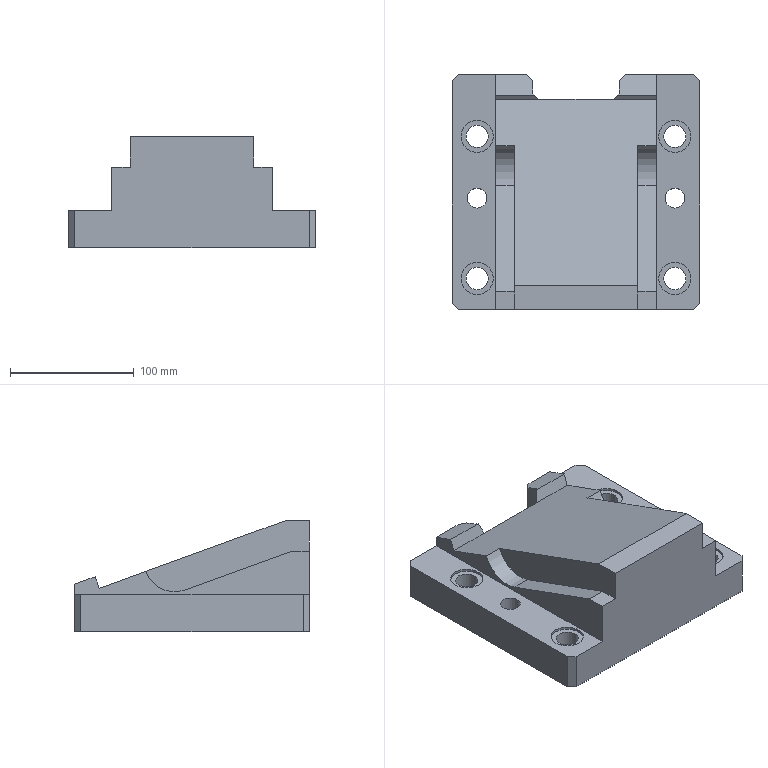Part | NX | features solid 2 | 1 solid | 70 faces | box 200 x 190 x 90 mm | volume 1698344 mm3 | plane 58 | cylinder 12 | commonest cylinder face diameters 18 x4 26 x4 16 x2 50 x2